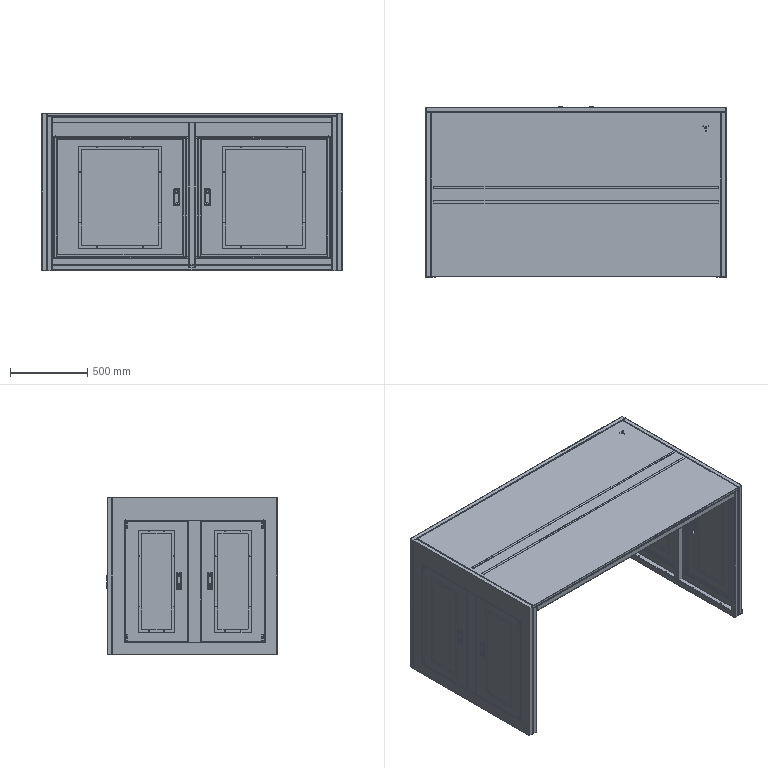Part | SolidWorks | features ReferencePattern 6, MirrorCompFeat 4 | 65 solids | 3884 faces | volume 22995452 mm3 | plane 2102 | cylinder 1430 | spline 280 | cone 72 | commonest cylinder face diameters 4 x427 1 x177 3 x126 8 x96 2 x90 5 x48